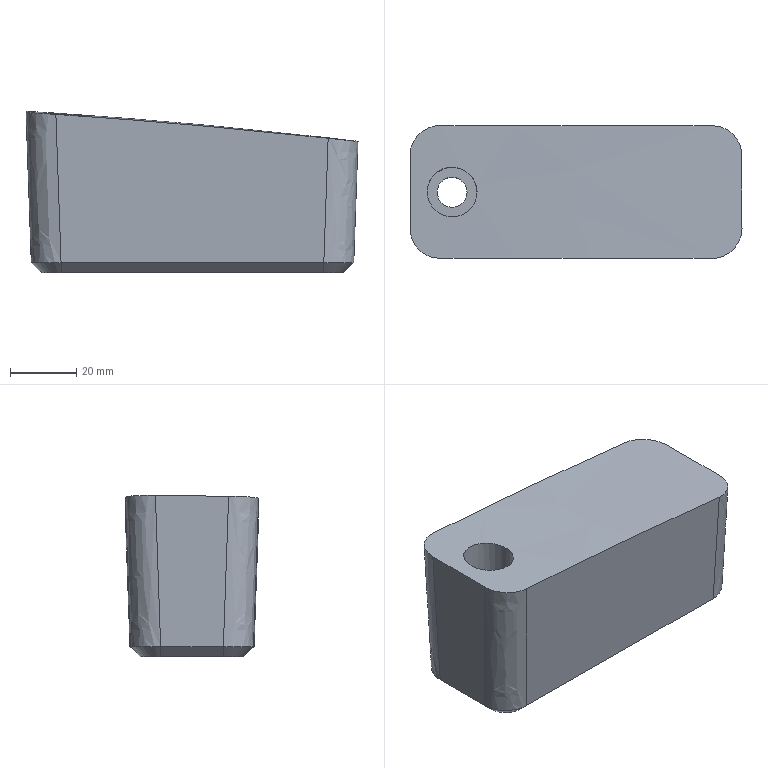Part | STEP file | solid 20 | 1 solid | 21 faces | box 99.984 x 40 x 48.51 mm | volume 156692 mm3 | spline 17 | plane 2 | cylinder 2 | commonest cylinder face diameters 9 x1 15 x1